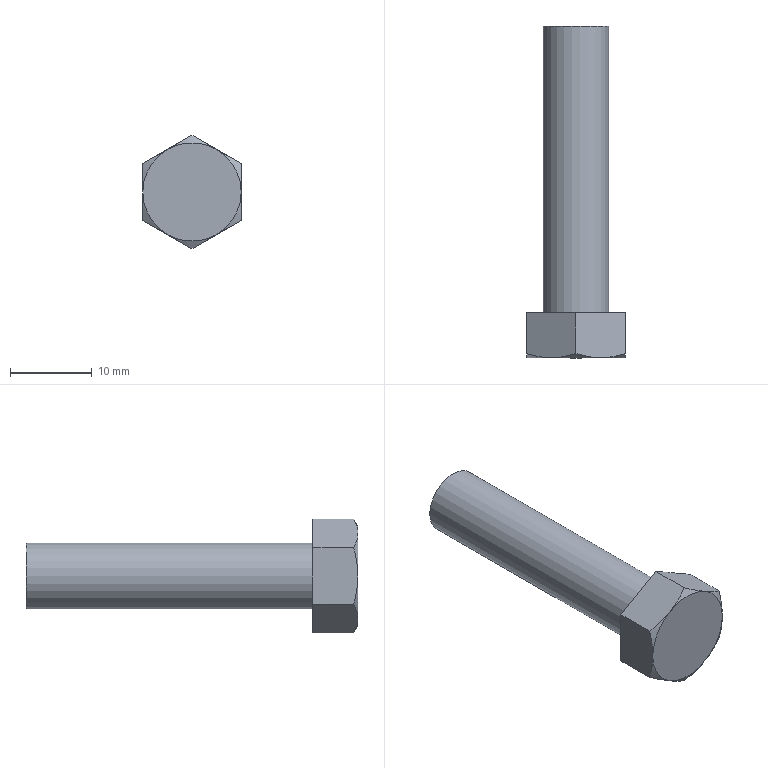Part | NX | features DATUM_CSYS 4, SKETCH 3, EXTRUDE 2, SWP104 1, SYMBOLIC_THREAD 1, UNITE 1 | 1 solid | 16 faces | box 12 x 40.5 x 13.856 mm | volume 2443 mm3 | plane 9 | cone 6 | cylinder 1 | commonest cylinder face diameters 8 x1
STEP:
#1=CARTESIAN_POINT('',(-6.,-4.964,-3.464));
#2=VERTEX_POINT('',#1);
#3=CARTESIAN_POINT('',(-6.,0.,-3.464));
#4=VERTEX_POINT('',#3);
#5=CARTESIAN_POINT('',(-6.,-5.5,-3.464));
#6=DIRECTION('',(0.,1.,0.));
#7=VECTOR('',#6,1000.);
#8=LINE('',#5,#7);
#9=EDGE_CURVE('',#2,#4,#8,.T.);
#10=ORIENTED_EDGE('',*,*,#9,.F.);
#11=CARTESIAN_POINT('',(-6.,-5.5,0.));
#12=VERTEX_POINT('',#11);
#13=CARTESIAN_POINT('',(-6.,-4.964,-3.464));
#14=CARTESIAN_POINT('',(-6.,-5.29,-2.336));
#15=CARTESIAN_POINT('',(-6.,-5.5,-1.172));
#16=CARTESIAN_POINT('',(-6.,-5.5,0.));
#17=B_SPLINE_CURVE_WITH_KNOTS('',3,(#13,#14,#15,#16),.UNSPECIFIED.,.F.,.F.,(4,4),(0.006361,0.009867),.UNSPECIFIED.);
#18=EDGE_CURVE('',#2,#12,#17,.T.);
#19=ORIENTED_EDGE('',*,*,#18,.T.);
#20=CARTESIAN_POINT('',(-6.,-4.964,3.464));
#21=VERTEX_POINT('',#20);
#22=CARTESIAN_POINT('',(-6.,-5.5,0.));
#23=CARTESIAN_POINT('',(-6.,-5.5,1.173));
#24=CARTESIAN_POINT('',(-6.,-5.288,2.344));
#25=CARTESIAN_POINT('',(-6.,-4.964,3.464));
#26=B_SPLINE_CURVE_WITH_KNOTS('',3,(#22,#23,#24,#25),.UNSPECIFIED.,.F.,.F.,(4,4),(0.009867,0.01338),.UNSPECIFIED.);
#27=EDGE_CURVE('',#12,#21,#26,.T.);
#28=ORIENTED_EDGE('',*,*,#27,.T.);
#29=CARTESIAN_POINT('',(-6.,0.,3.464));
#30=VERTEX_POINT('',#29);
#31=CARTESIAN_POINT('',(-6.,-5.5,3.464));
#32=DIRECTION('',(0.,1.,0.));
#33=VECTOR('',#32,1000.);
#34=LINE('',#31,#33);
#35=EDGE_CURVE('',#21,#30,#34,.T.);
#36=ORIENTED_EDGE('',*,*,#35,.T.);
#37=CARTESIAN_POINT('',(-6.,0.,3.464));
#38=DIRECTION('',(0.,0.,-1.));
#39=VECTOR('',#38,1000.);
#40=LINE('',#37,#39);
#41=EDGE_CURVE('',#30,#4,#40,.T.);
#42=ORIENTED_EDGE('',*,*,#41,.T.);
#43=EDGE_LOOP('',(#10,#19,#28,#36,#42));
#44=FACE_BOUND('',#43,.T.);
#45=CARTESIAN_POINT('',(-6.,-5.5,3.464));
#46=DIRECTION('',(1.,0.,0.));
#47=DIRECTION('',(0.,0.,-1.));
#48=AXIS2_PLACEMENT_3D('',#45,#46,#47);
#49=PLANE('',#48);
#50=ADVANCED_FACE('',(#44),#49,.F.);
#51=CARTESIAN_POINT('',(0.,-4.964,-6.928));
#52=VERTEX_POINT('',#51);
#53=CARTESIAN_POINT('',(0.,0.,-6.928));
#54=VERTEX_POINT('',#53);
#55=CARTESIAN_POINT('',(0.,-5.5,-6.928));
#56=DIRECTION('',(0.,1.,0.));
#57=VECTOR('',#56,1000.);
#58=LINE('',#55,#57);
#59=EDGE_CURVE('',#52,#54,#58,.T.);
#60=ORIENTED_EDGE('',*,*,#59,.F.);
#61=CARTESIAN_POINT('',(-3.,-5.5,-5.196));
#62=VERTEX_POINT('',#61);
#63=CARTESIAN_POINT('',(0.,-4.964,-6.928));
#64=CARTESIAN_POINT('',(-0.9815,-5.291,-6.362));
#65=CARTESIAN_POINT('',(-1.978,-5.5,-5.786));
#66=CARTESIAN_POINT('',(-3.,-5.5,-5.196));
#67=B_SPLINE_CURVE_WITH_KNOTS('',3,(#63,#64,#65,#66),.UNSPECIFIED.,.F.,.F.,(4,4),(0.000000238,0.003505),.UNSPECIFIED.);
#68=EDGE_CURVE('',#52,#62,#67,.T.);
#69=ORIENTED_EDGE('',*,*,#68,.T.);
#70=CARTESIAN_POINT('',(-3.,-5.5,-5.196));
#71=CARTESIAN_POINT('',(-4.018,-5.5,-4.608));
#72=CARTESIAN_POINT('',(-5.021,-5.29,-4.029));
#73=CARTESIAN_POINT('',(-6.,-4.964,-3.464));
#74=B_SPLINE_CURVE_WITH_KNOTS('',3,(#70,#71,#72,#73),.UNSPECIFIED.,.F.,.F.,(4,4),(0.003505,0.006997),.UNSPECIFIED.);
#75=EDGE_CURVE('',#62,#2,#74,.T.);
#76=ORIENTED_EDGE('',*,*,#75,.T.);
#77=ORIENTED_EDGE('',*,*,#9,.T.);
#78=CARTESIAN_POINT('',(-6.,0.,-3.464));
#79=DIRECTION('',(0.866,0.,-0.5));
#80=VECTOR('',#79,1000.);
#81=LINE('',#78,#80);
#82=EDGE_CURVE('',#4,#54,#81,.T.);
#83=ORIENTED_EDGE('',*,*,#82,.T.);
#84=EDGE_LOOP('',(#60,#69,#76,#77,#83));
#85=FACE_BOUND('',#84,.T.);
#86=CARTESIAN_POINT('',(-6.,-5.5,-3.464));
#87=DIRECTION('',(0.5,0.,0.866));
#88=DIRECTION('',(0.866,0.,-0.5));
#89=AXIS2_PLACEMENT_3D('',#86,#87,#88);
#90=PLANE('',#89);
#91=ADVANCED_FACE('',(#85),#90,.F.);
#92=CARTESIAN_POINT('',(6.,-4.964,-3.464));
#93=VERTEX_POINT('',#92);
#94=CARTESIAN_POINT('',(6.,0.,-3.464));
#95=VERTEX_POINT('',#94);
#96=CARTESIAN_POINT('',(6.,-5.5,-3.464));
#97=DIRECTION('',(0.,1.,0.));
#98=VECTOR('',#97,1000.);
#99=LINE('',#96,#98);
#100=EDGE_CURVE('',#93,#95,#99,.T.);
#101=ORIENTED_EDGE('',*,*,#100,.F.);
#102=CARTESIAN_POINT('',(3.,-5.5,-5.196));
#103=VERTEX_POINT('',#102);
#104=CARTESIAN_POINT('',(6.,-4.964,-3.464));
#105=CARTESIAN_POINT('',(5.018,-5.291,-4.031));
#106=CARTESIAN_POINT('',(4.022,-5.5,-4.606));
#107=CARTESIAN_POINT('',(3.,-5.5,-5.196));
#108=B_SPLINE_CURVE_WITH_KNOTS('',3,(#104,#105,#106,#107),.UNSPECIFIED.,.F.,.F.,(4,4),(0.000000238,0.003505),.UNSPECIFIED.);
#109=EDGE_CURVE('',#93,#103,#108,.T.);
#110=ORIENTED_EDGE('',*,*,#109,.T.);
#111=CARTESIAN_POINT('',(3.,-5.5,-5.196));
#112=CARTESIAN_POINT('',(1.982,-5.5,-5.784));
#113=CARTESIAN_POINT('',(0.9791,-5.29,-6.363));
#114=CARTESIAN_POINT('',(0.,-4.964,-6.928));
#115=B_SPLINE_CURVE_WITH_KNOTS('',3,(#111,#112,#113,#114),.UNSPECIFIED.,.F.,.F.,(4,4),(0.003505,0.006997),.UNSPECIFIED.);
#116=EDGE_CURVE('',#103,#52,#115,.T.);
#117=ORIENTED_EDGE('',*,*,#116,.T.);
#118=ORIENTED_EDGE('',*,*,#59,.T.);
#119=CARTESIAN_POINT('',(0.,0.,-6.928));
#120=DIRECTION('',(0.866,0.,0.5));
#121=VECTOR('',#120,1000.);
#122=LINE('',#119,#121);
#123=EDGE_CURVE('',#54,#95,#122,.T.);
#124=ORIENTED_EDGE('',*,*,#123,.T.);
#125=EDGE_LOOP('',(#101,#110,#117,#118,#124));
#126=FACE_BOUND('',#125,.T.);
#127=CARTESIAN_POINT('',(0.,-5.5,-6.928));
#128=DIRECTION('',(-0.5,0.,0.866));
#129=DIRECTION('',(0.866,0.,0.5));
#130=AXIS2_PLACEMENT_3D('',#127,#128,#129);
#131=PLANE('',#130);
#132=ADVANCED_FACE('',(#126),#131,.F.);
#133=CARTESIAN_POINT('',(6.,-4.964,3.464));
#134=VERTEX_POINT('',#133);
#135=CARTESIAN_POINT('',(6.,0.,3.464));
#136=VERTEX_POINT('',#135);
#137=CARTESIAN_POINT('',(6.,-5.5,3.464));
#138=DIRECTION('',(0.,1.,0.));
#139=VECTOR('',#138,1000.);
#140=LINE('',#137,#139);
#141=EDGE_CURVE('',#134,#136,#140,.T.);
#142=ORIENTED_EDGE('',*,*,#141,.F.);
#143=CARTESIAN_POINT('',(6.,-5.5,0.));
#144=VERTEX_POINT('',#143);
#145=CARTESIAN_POINT('',(6.,-5.5,0.));
#146=CARTESIAN_POINT('',(6.,-5.5,1.173));
#147=CARTESIAN_POINT('',(6.,-5.288,2.344));
#148=CARTESIAN_POINT('',(6.,-4.964,3.464));
#149=B_SPLINE_CURVE_WITH_KNOTS('',3,(#145,#146,#147,#148),.UNSPECIFIED.,.F.,.F.,(4,4),(0.009867,0.01338),.UNSPECIFIED.);
#150=EDGE_CURVE('',#134,#144,#149,.F.);
#151=ORIENTED_EDGE('',*,*,#150,.T.);
#152=CARTESIAN_POINT('',(6.,-4.964,-3.464));
#153=CARTESIAN_POINT('',(6.,-5.29,-2.336));
#154=CARTESIAN_POINT('',(6.,-5.5,-1.172));
#155=CARTESIAN_POINT('',(6.,-5.5,0.));
#156=B_SPLINE_CURVE_WITH_KNOTS('',3,(#152,#153,#154,#155),.UNSPECIFIED.,.F.,.F.,(4,4),(0.006361,0.009867),.UNSPECIFIED.);
#157=EDGE_CURVE('',#144,#93,#156,.F.);
#158=ORIENTED_EDGE('',*,*,#157,.T.);
#159=ORIENTED_EDGE('',*,*,#100,.T.);
#160=CARTESIAN_POINT('',(6.,0.,-3.464));
#161=DIRECTION('',(0.,0.,1.));
#162=VECTOR('',#161,1000.);
#163=LINE('',#160,#162);
#164=EDGE_CURVE('',#95,#136,#163,.T.);
#165=ORIENTED_EDGE('',*,*,#164,.T.);
#166=EDGE_LOOP('',(#142,#151,#158,#159,#165));
#167=FACE_BOUND('',#166,.T.);
#168=CARTESIAN_POINT('',(6.,-5.5,-3.464));
#169=DIRECTION('',(-1.,0.,0.));
#170=DIRECTION('',(0.,0.,1.));
#171=AXIS2_PLACEMENT_3D('',#168,#169,#170);
#172=PLANE('',#171);
#173=ADVANCED_FACE('',(#167),#172,.F.);
#174=CARTESIAN_POINT('',(0.,-4.964,6.928));
#175=VERTEX_POINT('',#174);
#176=CARTESIAN_POINT('',(0.,0.,6.928));
#177=VERTEX_POINT('',#176);
#178=CARTESIAN_POINT('',(0.,-5.5,6.928));
#179=DIRECTION('',(0.,1.,0.));
#180=VECTOR('',#179,1000.);
#181=LINE('',#178,#180);
#182=EDGE_CURVE('',#175,#177,#181,.T.);
#183=ORIENTED_EDGE('',*,*,#182,.F.);
#184=CARTESIAN_POINT('',(3.,-5.5,5.196));
#185=VERTEX_POINT('',#184);
#186=CARTESIAN_POINT('',(0.,-4.964,6.928));
#187=CARTESIAN_POINT('',(0.9815,-5.291,6.362));
#188=CARTESIAN_POINT('',(1.978,-5.5,5.786));
#189=CARTESIAN_POINT('',(3.,-5.5,5.196));
#190=B_SPLINE_CURVE_WITH_KNOTS('',3,(#186,#187,#188,#189),.UNSPECIFIED.,.F.,.F.,(4,4),(0.000000238,0.003505),.UNSPECIFIED.);
#191=EDGE_CURVE('',#175,#185,#190,.T.);
#192=ORIENTED_EDGE('',*,*,#191,.T.);
#193=CARTESIAN_POINT('',(3.,-5.5,5.196));
#194=CARTESIAN_POINT('',(4.018,-5.5,4.608));
#195=CARTESIAN_POINT('',(5.021,-5.29,4.029));
#196=CARTESIAN_POINT('',(6.,-4.964,3.464));
#197=B_SPLINE_CURVE_WITH_KNOTS('',3,(#193,#194,#195,#196),.UNSPECIFIED.,.F.,.F.,(4,4),(0.003505,0.006997),.UNSPECIFIED.);
#198=EDGE_CURVE('',#185,#134,#197,.T.);
#199=ORIENTED_EDGE('',*,*,#198,.T.);
#200=ORIENTED_EDGE('',*,*,#141,.T.);
#201=CARTESIAN_POINT('',(6.,0.,3.464));
#202=DIRECTION('',(-0.866,0.,0.5));
#203=VECTOR('',#202,1000.);
#204=LINE('',#201,#203);
#205=EDGE_CURVE('',#136,#177,#204,.T.);
#206=ORIENTED_EDGE('',*,*,#205,.T.);
#207=EDGE_LOOP('',(#183,#192,#199,#200,#206));
#208=FACE_BOUND('',#207,.T.);
#209=CARTESIAN_POINT('',(6.,-5.5,3.464));
#210=DIRECTION('',(-0.5,0.,-0.866));
#211=DIRECTION('',(-0.866,0.,0.5));
#212=AXIS2_PLACEMENT_3D('',#209,#210,#211);
#213=PLANE('',#212);
#214=ADVANCED_FACE('',(#208),#213,.F.);
#215=ORIENTED_EDGE('',*,*,#35,.F.);
#216=CARTESIAN_POINT('',(-3.,-5.5,5.196));
#217=VERTEX_POINT('',#216);
#218=CARTESIAN_POINT('',(-6.,-4.964,3.464));
#219=CARTESIAN_POINT('',(-5.018,-5.291,4.031));
#220=CARTESIAN_POINT('',(-4.022,-5.5,4.606));
#221=CARTESIAN_POINT('',(-3.,-5.5,5.196));
#222=B_SPLINE_CURVE_WITH_KNOTS('',3,(#218,#219,#220,#221),.UNSPECIFIED.,.F.,.F.,(4,4),(0.000000238,0.003505),.UNSPECIFIED.);
#223=EDGE_CURVE('',#21,#217,#222,.T.);
#224=ORIENTED_EDGE('',*,*,#223,.T.);
#225=CARTESIAN_POINT('',(-3.,-5.5,5.196));
#226=CARTESIAN_POINT('',(-1.982,-5.5,5.784));
#227=CARTESIAN_POINT('',(-0.9791,-5.29,6.363));
#228=CARTESIAN_POINT('',(0.,-4.964,6.928));
#229=B_SPLINE_CURVE_WITH_KNOTS('',3,(#225,#226,#227,#228),.UNSPECIFIED.,.F.,.F.,(4,4),(0.003505,0.006997),.UNSPECIFIED.);
#230=EDGE_CURVE('',#217,#175,#229,.T.);
#231=ORIENTED_EDGE('',*,*,#230,.T.);
#232=ORIENTED_EDGE('',*,*,#182,.T.);
#233=CARTESIAN_POINT('',(0.,0.,6.928));
#234=DIRECTION('',(-0.866,0.,-0.5));
#235=VECTOR('',#234,1000.);
#236=LINE('',#233,#235);
#237=EDGE_CURVE('',#177,#30,#236,.T.);
#238=ORIENTED_EDGE('',*,*,#237,.T.);
#239=EDGE_LOOP('',(#215,#224,#231,#232,#238));
#240=FACE_BOUND('',#239,.T.);
#241=CARTESIAN_POINT('',(0.,-5.5,6.928));
#242=DIRECTION('',(0.5,0.,-0.866));
#243=DIRECTION('',(-0.866,0.,-0.5));
#244=AXIS2_PLACEMENT_3D('',#241,#242,#243);
#245=PLANE('',#244);
#246=ADVANCED_FACE('',(#240),#245,.F.);
#247=CARTESIAN_POINT('',(4.,0.,0.));
#248=VERTEX_POINT('',#247);
#249=CARTESIAN_POINT('',(0.,0.,0.));
#250=DIRECTION('',(0.,-1.,0.));
#251=DIRECTION('',(1.,0.,0.));
#252=AXIS2_PLACEMENT_3D('',#249,#250,#251);
#253=CIRCLE('',#252,4.);
#254=EDGE_CURVE('',#248,#248,#253,.T.);
#255=ORIENTED_EDGE('',*,*,#254,.T.);
#256=EDGE_LOOP('',(#255));
#257=FACE_BOUND('',#256,.T.);
#258=ORIENTED_EDGE('',*,*,#41,.F.);
#259=ORIENTED_EDGE('',*,*,#237,.F.);
#260=ORIENTED_EDGE('',*,*,#205,.F.);
#261=ORIENTED_EDGE('',*,*,#164,.F.);
#262=ORIENTED_EDGE('',*,*,#123,.F.);
#263=ORIENTED_EDGE('',*,*,#82,.F.);
#264=EDGE_LOOP('',(#258,#259,#260,#261,#262,#263));
#265=FACE_BOUND('',#264,.T.);
#266=CARTESIAN_POINT('',(0.,0.,0.));
#267=DIRECTION('',(0.,-1.,0.));
#268=DIRECTION('',(0.,0.,-1.));
#269=AXIS2_PLACEMENT_3D('',#266,#267,#268);
#270=PLANE('',#269);
#271=ADVANCED_FACE('',(#257,#265),#270,.F.);
#272=ORIENTED_EDGE('',*,*,#230,.F.);
#273=CARTESIAN_POINT('',(0.,-5.5,0.));
#274=DIRECTION('',(0.,-1.,0.));
#275=DIRECTION('',(0.,0.,-1.));
#276=AXIS2_PLACEMENT_3D('',#273,#274,#275);
#277=CIRCLE('',#276,6.);
#278=EDGE_CURVE('',#185,#217,#277,.T.);
#279=ORIENTED_EDGE('',*,*,#278,.F.);
#280=ORIENTED_EDGE('',*,*,#191,.F.);
#281=EDGE_LOOP('',(#272,#279,#280));
#282=FACE_BOUND('',#281,.T.);
#283=CARTESIAN_POINT('',(0.,-3.8,0.));
#284=DIRECTION('',(0.,1.,0.));
#285=DIRECTION('',(0.,0.,1.));
#286=AXIS2_PLACEMENT_3D('',#283,#284,#285);
#287=CONICAL_SURFACE('',#286,8.944,1.047);
#288=ADVANCED_FACE('',(#282),#287,.T.);
#289=CARTESIAN_POINT('',(0.,-5.5,0.));
#290=DIRECTION('',(0.,-1.,0.));
#291=DIRECTION('',(0.,0.,-1.));
#292=AXIS2_PLACEMENT_3D('',#289,#290,#291);
#293=CIRCLE('',#292,6.);
#294=EDGE_CURVE('',#217,#12,#293,.T.);
#295=ORIENTED_EDGE('',*,*,#294,.F.);
#296=ORIENTED_EDGE('',*,*,#223,.F.);
#297=ORIENTED_EDGE('',*,*,#27,.F.);
#298=EDGE_LOOP('',(#295,#296,#297));
#299=FACE_BOUND('',#298,.T.);
#300=CARTESIAN_POINT('',(0.,-3.8,0.));
#301=DIRECTION('',(0.,1.,0.));
#302=DIRECTION('',(0.,0.,1.));
#303=AXIS2_PLACEMENT_3D('',#300,#301,#302);
#304=CONICAL_SURFACE('',#303,8.944,1.047);
#305=ADVANCED_FACE('',(#299),#304,.T.);
#306=ORIENTED_EDGE('',*,*,#198,.F.);
#307=CARTESIAN_POINT('',(0.,-5.5,0.));
#308=DIRECTION('',(0.,-1.,0.));
#309=DIRECTION('',(0.,0.,-1.));
#310=AXIS2_PLACEMENT_3D('',#307,#308,#309);
#311=CIRCLE('',#310,6.);
#312=EDGE_CURVE('',#144,#185,#311,.T.);
#313=ORIENTED_EDGE('',*,*,#312,.F.);
#314=ORIENTED_EDGE('',*,*,#150,.F.);
#315=EDGE_LOOP('',(#306,#313,#314));
#316=FACE_BOUND('',#315,.T.);
#317=CARTESIAN_POINT('',(0.,-3.8,0.));
#318=DIRECTION('',(0.,1.,0.));
#319=DIRECTION('',(0.,0.,1.));
#320=AXIS2_PLACEMENT_3D('',#317,#318,#319);
#321=CONICAL_SURFACE('',#320,8.944,1.047);
#322=ADVANCED_FACE('',(#316),#321,.T.);
#323=ORIENTED_EDGE('',*,*,#157,.F.);
#324=CARTESIAN_POINT('',(0.,-5.5,0.));
#325=DIRECTION('',(0.,-1.,0.));
#326=DIRECTION('',(0.,0.,-1.));
#327=AXIS2_PLACEMENT_3D('',#324,#325,#326);
#328=CIRCLE('',#327,6.);
#329=EDGE_CURVE('',#103,#144,#328,.T.);
#330=ORIENTED_EDGE('',*,*,#329,.F.);
#331=ORIENTED_EDGE('',*,*,#109,.F.);
#332=EDGE_LOOP('',(#323,#330,#331));
#333=FACE_BOUND('',#332,.T.);
#334=CARTESIAN_POINT('',(0.,-3.8,0.));
#335=DIRECTION('',(0.,1.,0.));
#336=DIRECTION('',(0.,0.,1.));
#337=AXIS2_PLACEMENT_3D('',#334,#335,#336);
#338=CONICAL_SURFACE('',#337,8.944,1.047);
#339=ADVANCED_FACE('',(#333),#338,.T.);
#340=CARTESIAN_POINT('',(0.,-5.5,0.));
#341=DIRECTION('',(0.,-1.,0.));
#342=DIRECTION('',(0.,0.,-1.));
#343=AXIS2_PLACEMENT_3D('',#340,#341,#342);
#344=CIRCLE('',#343,6.);
#345=EDGE_CURVE('',#62,#103,#344,.T.);
#346=ORIENTED_EDGE('',*,*,#345,.F.);
#347=ORIENTED_EDGE('',*,*,#68,.F.);
#348=ORIENTED_EDGE('',*,*,#116,.F.);
#349=EDGE_LOOP('',(#346,#347,#348));
#350=FACE_BOUND('',#349,.T.);
#351=CARTESIAN_POINT('',(0.,-3.8,0.));
#352=DIRECTION('',(0.,1.,0.));
#353=DIRECTION('',(0.,0.,1.));
#354=AXIS2_PLACEMENT_3D('',#351,#352,#353);
#355=CONICAL_SURFACE('',#354,8.944,1.047);
#356=ADVANCED_FACE('',(#350),#355,.T.);
#357=CARTESIAN_POINT('',(0.,-5.5,0.));
#358=DIRECTION('',(0.,-1.,0.));
#359=DIRECTION('',(0.,0.,-1.));
#360=AXIS2_PLACEMENT_3D('',#357,#358,#359);
#361=CIRCLE('',#360,6.);
#362=EDGE_CURVE('',#12,#62,#361,.T.);
#363=ORIENTED_EDGE('',*,*,#362,.F.);
#364=ORIENTED_EDGE('',*,*,#18,.F.);
#365=ORIENTED_EDGE('',*,*,#75,.F.);
#366=EDGE_LOOP('',(#363,#364,#365));
#367=FACE_BOUND('',#366,.T.);
#368=CARTESIAN_POINT('',(0.,-3.8,0.));
#369=DIRECTION('',(0.,1.,0.));
#370=DIRECTION('',(0.,0.,1.));
#371=AXIS2_PLACEMENT_3D('',#368,#369,#370);
#372=CONICAL_SURFACE('',#371,8.944,1.047);
#373=ADVANCED_FACE('',(#367),#372,.T.);
#374=ORIENTED_EDGE('',*,*,#345,.T.);
#375=ORIENTED_EDGE('',*,*,#329,.T.);
#376=ORIENTED_EDGE('',*,*,#312,.T.);
#377=ORIENTED_EDGE('',*,*,#278,.T.);
#378=ORIENTED_EDGE('',*,*,#294,.T.);
#379=ORIENTED_EDGE('',*,*,#362,.T.);
#380=EDGE_LOOP('',(#374,#375,#376,#377,#378,#379));
#381=FACE_BOUND('',#380,.T.);
#382=CARTESIAN_POINT('',(0.,-5.5,0.));
#383=DIRECTION('',(0.,-1.,0.));
#384=DIRECTION('',(0.,0.,-1.));
#385=AXIS2_PLACEMENT_3D('',#382,#383,#384);
#386=PLANE('',#385);
#387=ADVANCED_FACE('',(#381),#386,.T.);
#388=CARTESIAN_POINT('',(4.,35.,0.));
#389=VERTEX_POINT('',#388);
#390=CARTESIAN_POINT('',(0.,35.,0.));
#391=DIRECTION('',(0.,-1.,0.));
#392=DIRECTION('',(1.,0.,0.));
#393=AXIS2_PLACEMENT_3D('',#390,#391,#392);
#394=CIRCLE('',#393,4.);
#395=EDGE_CURVE('',#389,#389,#394,.T.);
#396=ORIENTED_EDGE('',*,*,#395,.T.);
#397=EDGE_LOOP('',(#396));
#398=FACE_BOUND('',#397,.T.);
#399=ORIENTED_EDGE('',*,*,#254,.F.);
#400=EDGE_LOOP('',(#399));
#401=FACE_BOUND('',#400,.T.);
#402=CARTESIAN_POINT('',(0.,35.,0.));
#403=DIRECTION('',(0.,-1.,0.));
#404=DIRECTION('',(0.,0.,-1.));
#405=AXIS2_PLACEMENT_3D('',#402,#403,#404);
#406=CYLINDRICAL_SURFACE('',#405,4.);
#407=ADVANCED_FACE('',(#398,#401),#406,.T.);
#408=ORIENTED_EDGE('',*,*,#395,.F.);
#409=EDGE_LOOP('',(#408));
#410=FACE_BOUND('',#409,.T.);
#411=CARTESIAN_POINT('',(0.,35.,0.));
#412=DIRECTION('',(0.,-1.,0.));
#413=DIRECTION('',(0.,0.,-1.));
#414=AXIS2_PLACEMENT_3D('',#411,#412,#413);
#415=PLANE('',#414);
#416=ADVANCED_FACE('',(#410),#415,.F.);
#417=CLOSED_SHELL('',(#50,#91,#132,#173,#214,#246,#271,#288,#305,#322,#339,#356,#373,#387,#407,#416));
#418=MANIFOLD_SOLID_BREP('',#417);
#419=(LENGTH_UNIT()NAMED_UNIT(*)SI_UNIT(.MILLI.,.METRE.));
#420=UNCERTAINTY_MEASURE_WITH_UNIT(LENGTH_MEASURE(0.0508),#419,'','');
#421=(NAMED_UNIT(*)PLANE_ANGLE_UNIT()SI_UNIT($,.RADIAN.));
#422=(NAMED_UNIT(*)SI_UNIT($,.STERADIAN.)SOLID_ANGLE_UNIT());
#423=(GEOMETRIC_REPRESENTATION_CONTEXT(3)GLOBAL_UNCERTAINTY_ASSIGNED_CONTEXT((#420))GLOBAL_UNIT_ASSIGNED_CONTEXT((#419,#421,#422))REPRESENTATION_CONTEXT('',''));
#424=ADVANCED_BREP_SHAPE_REPRESENTATION('',(#418),#423);